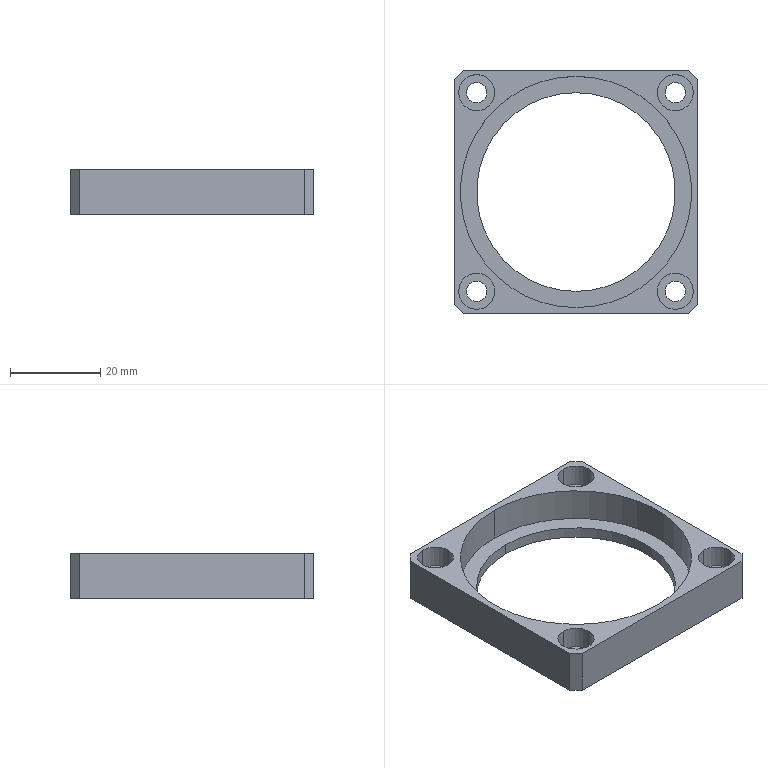NC program | NX | posted with a generic post | part box 54 x 54 x 10 mm
Whole program:
N10 G17 G21 G94 G90
(DRILLING , TOOL : D6A45)
N12 T07 M6
N14 G54
N16 G17 G0 G90 X22. Y-22. S5000 M3
N18 G43 Z30. H7
N20 G94 G81 G98 Z-1. F250. R3.
N22 Y22.
N24 X-22.
N26 X0. Y0.
N28 X-22. Y-22.
N30 G80
N32 G0 X-22. Y-22. Z30.
N34 M5
(DRILLING_COPY , TOOL : 4.5ZT)
N36 T14 M6
N38 G54
N40 G17 G0 G90 X22. Y-22. S2000 M3
N42 G43 Z30. H14
N44 G94 G83 G98 Z-12.852 F250. Q2. R3.
N46 Y22.
N48 X-22.
N50 X0. Y0.
N52 X-22. Y-22.
N54 G80
N56 G0 X-22. Y-22. Z30.
N58 M5
(HOLE_MILLING , TOOL : D6)
N60 T06 M6
N62 G54
N64 G17 G0 G90 X-22. Y22. S9500 M3
N66 G43 Z30. H6
N68 Z0.6
N70 G94 G3 X-21.5 Y21.5 R0.5 F1500.
N72 X-21. Y22. R0.5
N74 X-21. Y22. Z0.1 I-1. J0.
N76 X-21. Y22. Z-0.4 I-1. J0.
N78 X-21. Y22. Z-0.9 I-1. J0.
N80 X-21. Y22. Z-1.4 I-1. J0.
N82 X-21. Y22. Z-1.9 I-1. J0.
N84 X-21. Y22. Z-2.4 I-1. J0.
N86 X-21. Y22. Z-2.9 I-1. J0.
N88 X-21. Y22. Z-3.4 I-1. J0.
N90 X-21. Y22. Z-3.9 I-1. J0.
N92 X-21. Y22. Z-4.4 I-1. J0.
N94 X-21. Y22. Z-4.9 I-1. J0.
N96 X-21.691 Y22.951 Z-5. R1.
N98 X-22.951 Y22.309 R1.
N100 X-21.691 Y22.951 R-1.
N102 X-22.321 Y22.63 R0.5
N104 X-22. Y22. R0.5
N106 G0 Z30.
N108 X22.
N110 Z0.6
N112 G3 X22.5 Y21.5 R0.5
N114 X23. Y22. R0.5
N116 X23. Y22. Z0.1 I-1. J0.
N118 X23. Y22. Z-0.4 I-1. J0.
N120 X23. Y22. Z-0.9 I-1. J0.
N122 X23. Y22. Z-1.4 I-1. J0.
N124 X23. Y22. Z-1.9 I-1. J0.
N126 X23. Y22. Z-2.4 I-1. J0.
N128 X23. Y22. Z-2.9 I-1. J0.
N130 X23. Y22. Z-3.4 I-1. J0.
N132 X23. Y22. Z-3.9 I-1. J0.
N134 X23. Y22. Z-4.4 I-1. J0.
N136 X23. Y22. Z-4.9 I-1. J0.
N138 X22.309 Y22.951 Z-5. R1.
N140 X21.049 Y22.309 R1.
N142 X22.309 Y22.951 R-1.
N144 X21.679 Y22.63 R0.5
N146 X22. Y22. R0.5
N148 G0 Z30.
N150 Y-22.
N152 Z0.6
N154 G3 X22.5 Y-22.5 R0.5
N156 X23. Y-22. R0.5
N158 X23. Y-22. Z0.1 I-1. J0.
N160 X23. Y-22. Z-0.4 I-1. J0.
N162 X23. Y-22. Z-0.9 I-1. J0.
N164 X23. Y-22. Z-1.4 I-1. J0.
N166 X23. Y-22. Z-1.9 I-1. J0.
N168 X23. Y-22. Z-2.4 I-1. J0.
N170 X23. Y-22. Z-2.9 I-1. J0.
N172 X23. Y-22. Z-3.4 I-1. J0.
N174 X23. Y-22. Z-3.9 I-1. J0.
N176 X23. Y-22. Z-4.4 I-1. J0.
N178 X23. Y-22. Z-4.9 I-1. J0.
N180 X22.309 Y-21.049 Z-5. R1.
N182 X21.049 Y-21.691 R1.
N184 X22.309 Y-21.049 R-1.
N186 X21.679 Y-21.37 R0.5
N188 X22. Y-22. R0.5
N190 G0 Z30.
N192 X-22.
N194 Z0.6
N196 G3 X-21.5 Y-22.5 R0.5
N198 X-21. Y-22. R0.5
N200 X-21. Y-22. Z0.1 I-1. J0.
N202 X-21. Y-22. Z-0.4 I-1. J0.
N204 X-21. Y-22. Z-0.9 I-1. J0.
N206 X-21. Y-22. Z-1.4 I-1. J0.
N208 X-21. Y-22. Z-1.9 I-1. J0.
N210 X-21. Y-22. Z-2.4 I-1. J0.
N212 X-21. Y-22. Z-2.9 I-1. J0.
N214 X-21. Y-22. Z-3.4 I-1. J0.
N216 X-21. Y-22. Z-3.9 I-1. J0.
N218 X-21. Y-22. Z-4.4 I-1. J0.
N220 X-21. Y-22. Z-4.9 I-1. J0.
N222 X-21.691 Y-21.049 Z-5. R1.
N224 X-22.951 Y-21.691 R1.
N226 X-21.691 Y-21.049 R-1.
N228 X-22.321 Y-21.37 R0.5
N230 X-22. Y-22. R0.5
N232 G0 Z30.
N234 M5
(HOLE_MILLING_COPY , TOOL : D10)
N236 T10 M6
N238 G54
N240 G17 G0 G90 X0. Y0. S9500 M3
N242 G43 Z30. H10
N244 Z0.6
N246 G94 G3 X2.563 Y-2.563 R2.562 F2200.
N248 X5.125 Y0. R2.562
N250 X5.125 Y0. Z0.1 I-5.125 J0.
N252 X5.125 Y0. Z-0.4 I-5.125 J0.
N254 X5.125 Y0. Z-0.9 I-5.125 J0.
N256 X5.125 Y0. Z-1.4 I-5.125 J0.
N258 X5.125 Y0. Z-1.9 I-5.125 J0.
N260 X5.125 Y0. Z-2.4 I-5.125 J0.
N262 X5.125 Y0. Z-2.9 I-5.125 J0.
N264 X5.125 Y0. Z-3.4 I-5.125 J0.
N266 X5.125 Y0. Z-3.9 I-5.125 J0.
N268 X5.125 Y0. Z-4.4 I-5.125 J0.
N270 X5.125 Y0. Z-4.9 I-5.125 J0.
N272 X5.125 Y0. Z-5.4 I-5.125 J0.
N274 X5.125 Y0. Z-5.9 I-5.125 J0.
N276 X5.125 Y0. Z-6.4 I-5.125 J0.
N278 X5.125 Y0. Z-6.9 I-5.125 J0.
N280 X5.125 Y0. Z-7.4 I-5.125 J0.
N282 X1.584 Y4.874 Z-7.5 R5.125
N284 X-4.874 Y1.584 R5.125
N286 X1.584 Y4.874 R-5.125
N288 X-1.645 Y3.229 R2.563
N290 X0. Y0. R2.563
N292 G0 Z0.6
N294 G3 X5.125 Y-5.125 R5.125
N296 X10.25 Y0. R5.125
N298 X10.25 Y0. Z0.1 I-10.25 J0.
N300 X10.25 Y0. Z-0.4 I-10.25 J0.
N302 X10.25 Y0. Z-0.9 I-10.25 J0.
N304 X10.25 Y0. Z-1.4 I-10.25 J0.
N306 X10.25 Y0. Z-1.9 I-10.25 J0.
N308 X10.25 Y0. Z-2.4 I-10.25 J0.
N310 X10.25 Y0. Z-2.9 I-10.25 J0.
N312 X10.25 Y0. Z-3.4 I-10.25 J0.
N314 X10.25 Y0. Z-3.9 I-10.25 J0.
N316 X10.25 Y0. Z-4.4 I-10.25 J0.
N318 X10.25 Y0. Z-4.9 I-10.25 J0.
N320 X10.25 Y0. Z-5.4 I-10.25 J0.
N322 X10.25 Y0. Z-5.9 I-10.25 J0.
N324 X10.25 Y0. Z-6.4 I-10.25 J0.
N326 X10.25 Y0. Z-6.9 I-10.25 J0.
N328 X10.25 Y0. Z-7.4 I-10.25 J0.
N330 X3.167 Y9.748 Z-7.5 R10.25
N332 X-9.748 Y3.167 R10.25
N334 X3.167 Y9.748 R-10.25
N336 X-3.29 Y6.458 R5.125
N338 X0. Y0. R5.125
N340 G0 Z0.6
N342 G3 X7.688 Y-7.688 R7.688
N344 X15.375 Y0. R7.688
N346 X15.375 Y0. Z0.1 I-15.375 J0.
N348 X15.375 Y0. Z-0.4 I-15.375 J0.
N350 X15.375 Y0. Z-0.9 I-15.375 J0.
N352 X15.375 Y0. Z-1.4 I-15.375 J0.
N354 X15.375 Y0. Z-1.9 I-15.375 J0.
N356 X15.375 Y0. Z-2.4 I-15.375 J0.
N358 X15.375 Y0. Z-2.9 I-15.375 J0.
N360 X15.375 Y0. Z-3.4 I-15.375 J0.
N362 X15.375 Y0. Z-3.9 I-15.375 J0.
N364 X15.375 Y0. Z-4.4 I-15.375 J0.
N366 X15.375 Y0. Z-4.9 I-15.375 J0.
N368 X15.375 Y0. Z-5.4 I-15.375 J0.
N370 X15.375 Y0. Z-5.9 I-15.375 J0.
N372 X15.375 Y0. Z-6.4 I-15.375 J0.
N374 X15.375 Y0. Z-6.9 I-15.375 J0.
N376 X15.375 Y0. Z-7.4 I-15.375 J0.
N378 X4.751 Y14.622 Z-7.5 R15.375
N380 X-14.622 Y4.751 R15.375
N382 X4.751 Y14.622 R-15.375
N384 X-4.936 Y9.687 R7.688
N386 X0. Y0. R7.688
N388 G0 Z0.6
N390 G3 X10.25 Y-10.25 R10.25
N392 X20.5 Y0. R10.25
N394 X20.5 Y0. Z0.1 I-20.5 J0.
N396 X20.5 Y0. Z-0.4 I-20.5 J0.
N398 X20.5 Y0. Z-0.9 I-20.5 J0.
N400 X20.5 Y0. Z-1.4 I-20.5 J0.
N402 X20.5 Y0. Z-1.9 I-20.5 J0.
N404 X20.5 Y0. Z-2.4 I-20.5 J0.
N406 X20.5 Y0. Z-2.9 I-20.5 J0.
N408 X20.5 Y0. Z-3.4 I-20.5 J0.
N410 X20.5 Y0. Z-3.9 I-20.5 J0.
N412 X20.5 Y0. Z-4.4 I-20.5 J0.
N414 X20.5 Y0. Z-4.9 I-20.5 J0.
N416 X20.5 Y0. Z-5.4 I-20.5 J0.
N418 X20.5 Y0. Z-5.9 I-20.5 J0.
N420 X20.5 Y0. Z-6.4 I-20.5 J0.
N422 X20.5 Y0. Z-6.9 I-20.5 J0.
N424 X20.5 Y0. Z-7.4 I-20.5 J0.
N426 X6.335 Y19.497 Z-7.5 R20.5
N428 X-19.497 Y6.335 R20.5
N430 X6.335 Y19.497 R-20.5
N432 X-6.581 Y12.916 R10.25
N434 X0. Y0. R10.25
N436 G0 Z30.
(HOLE_MILLING_COPY_COPY , TOOL : D10)
N438 Z-6.9
N440 G3 X2.817 Y-2.817 R2.817
N442 X5.633 Y0. R2.817
N444 X5.633 Y0. Z-7.4 I-5.633 J0.
N446 X5.633 Y0. Z-7.9 I-5.633 J0.
N448 X5.633 Y0. Z-8.4 I-5.633 J0.
N450 X5.633 Y0. Z-8.9 I-5.633 J0.
N452 X5.633 Y0. Z-9.4 I-5.633 J0.
N454 X5.633 Y0. Z-9.9 I-5.633 J0.
N456 X1.741 Y5.358 Z-10. R5.633
N458 X-5.358 Y1.741 R5.633
N460 X1.741 Y5.358 R-5.633
N462 X-1.808 Y3.549 R2.817
N464 X0. Y0. R2.817
N466 G0 Z-6.9
N468 G3 X5.633 Y-5.633 R5.633
N470 X11.267 Y0. R5.633
N472 X11.267 Y0. Z-7.4 I-11.267 J0.
N474 X11.267 Y0. Z-7.9 I-11.267 J0.
N476 X11.267 Y0. Z-8.4 I-11.267 J0.
N478 X11.267 Y0. Z-8.9 I-11.267 J0.
N480 X11.267 Y0. Z-9.4 I-11.267 J0.
N482 X11.267 Y0. Z-9.9 I-11.267 J0.
N484 X3.482 Y10.715 Z-10. R11.267
N486 X-10.715 Y3.482 R11.267
N488 X3.482 Y10.715 R-11.267
N490 X-3.617 Y7.098 R5.633
N492 X0. Y0. R5.633
N494 G0 Z-6.9
N496 G3 X8.45 Y-8.45 R8.45
N498 X16.9 Y0. R8.45
N500 X16.9 Y0. Z-7.4 I-16.9 J0.
N502 X16.9 Y0. Z-7.9 I-16.9 J0.
N504 X16.9 Y0. Z-8.4 I-16.9 J0.
N506 X16.9 Y0. Z-8.9 I-16.9 J0.
N508 X16.9 Y0. Z-9.4 I-16.9 J0.
N510 X16.9 Y0. Z-9.9 I-16.9 J0.
N512 X5.222 Y16.073 Z-10. R16.9
N514 X-16.073 Y5.222 R16.9
N516 X5.222 Y16.073 R-16.9
N518 X-5.425 Y10.648 R8.45
N520 X0. Y0. R8.45
N522 G0 Z30.
(ZLEVEL_PROFILE , TOOL : D10)
N524 X2.109 Y-32.1
N526 Z1.5
N528 G1 X-25. Z0.079 F1000.
N530 X-25.554 Z0.05
N532 X-26.963 Y-31.74 Z-0.026
N534 X-28.215 Y-30.998 Z-0.102
N536 X-30.998 Y-28.215 Z-0.309
N538 X-31.74 Y-26.963 Z-0.385
N540 X-32.1 Y-25.554 Z-0.461
N542 Y-25. Z-0.49
N544 Y25. F2500.
N546 G2 X-30.606 Y28.606 R5.1
N548 G1 X-28.606 Y30.606
N550 G2 X-25. Y32.1 R5.1
N552 G1 X25.
N554 G2 X28.606 Y30.606 R5.1
N556 G1 X30.606 Y28.606
N558 G2 X32.1 Y25. R5.1
N560 G1 Y-25.
N562 G2 X30.606 Y-28.606 R5.1
N564 G1 X28.606 Y-30.606
N566 G2 X25. Y-32.1 R5.1
N568 G1 X-25.
N570 G2 X-28.606 Y-30.606 R5.1
N572 G1 X-30.606 Y-28.606
N574 G2 X-32.1 Y-25. R5.1
N576 G1 Y3.072 Z-0.98
N578 Y25.
N580 G2 X-30.606 Y28.606 R5.1
N582 G1 X-28.606 Y30.606
N584 G2 X-25. Y32.1 R5.1
N586 G1 X25.
N588 G2 X28.606 Y30.606 R5.1
N590 G1 X30.606 Y28.606
N592 G2 X32.1 Y25. R5.1
N594 G1 Y-25.
N596 G2 X30.606 Y-28.606 R5.1
N598 G1 X28.606 Y-30.606
N600 G2 X25. Y-32.1 R5.1
N602 G1 X-25.
N604 G2 X-28.606 Y-30.606 R5.1
N606 G1 X-30.606 Y-28.606
N608 G2 X-32.1 Y-25. R5.1
N610 G1 Y3.072 Z-1.47
N612 Y25.
N614 G2 X-30.606 Y28.606 R5.1
N616 G1 X-28.606 Y30.606
N618 G2 X-25. Y32.1 R5.1
N620 G1 X25.
N622 G2 X28.606 Y30.606 R5.1
N624 G1 X30.606 Y28.606
N626 G2 X32.1 Y25. R5.1
N628 G1 Y-25.
N630 G2 X30.606 Y-28.606 R5.1
N632 G1 X28.606 Y-30.606
N634 G2 X25. Y-32.1 R5.1
N636 G1 X-25.
N638 G2 X-28.606 Y-30.606 R5.1
N640 G1 X-30.606 Y-28.606
N642 G2 X-32.1 Y-25. R5.1
N644 G1 Y3.072 Z-1.96
N646 Y25.
N648 G2 X-30.606 Y28.606 R5.1
N650 G1 X-28.606 Y30.606
N652 G2 X-25. Y32.1 R5.1
N654 G1 X25.
N656 G2 X28.606 Y30.606 R5.1
N658 G1 X30.606 Y28.606
N660 G2 X32.1 Y25. R5.1
N662 G1 Y-25.
N664 G2 X30.606 Y-28.606 R5.1
N666 G1 X28.606 Y-30.606
N668 G2 X25. Y-32.1 R5.1
N670 G1 X-25.
N672 G2 X-28.606 Y-30.606 R5.1
N674 G1 X-30.606 Y-28.606
N676 G2 X-32.1 Y-25. R5.1
N678 G1 Y3.072 Z-2.45
N680 Y25.
N682 G2 X-30.606 Y28.606 R5.1
N684 G1 X-28.606 Y30.606
N686 G2 X-25. Y32.1 R5.1
N688 G1 X25.
N690 G2 X28.606 Y30.606 R5.1
N692 G1 X30.606 Y28.606
N694 G2 X32.1 Y25. R5.1
N696 G1 Y-25.
N698 G2 X30.606 Y-28.606 R5.1
N700 G1 X28.606 Y-30.606
N702 G2 X25. Y-32.1 R5.1
N704 G1 X-25.
N706 G2 X-28.606 Y-30.606 R5.1
N708 G1 X-30.606 Y-28.606
N710 G2 X-32.1 Y-25. R5.1
N712 G1 Y3.072 Z-2.94
N714 Y25.
N716 G2 X-30.606 Y28.606 R5.1
N718 G1 X-28.606 Y30.606
N720 G2 X-25. Y32.1 R5.1
N722 G1 X25.
N724 G2 X28.606 Y30.606 R5.1
N726 G1 X30.606 Y28.606
N728 G2 X32.1 Y25. R5.1
N730 G1 Y-25.
N732 G2 X30.606 Y-28.606 R5.1
N734 G1 X28.606 Y-30.606
N736 G2 X25. Y-32.1 R5.1
N738 G1 X-25.
N740 G2 X-28.606 Y-30.606 R5.1
N742 G1 X-30.606 Y-28.606
N744 G2 X-32.1 Y-25. R5.1
N746 G1 Y3.072 Z-3.43
N748 Y25.
N750 G2 X-30.606 Y28.606 R5.1
N752 G1 X-28.606 Y30.606
N754 G2 X-25. Y32.1 R5.1
N756 G1 X25.
N758 G2 X28.606 Y30.606 R5.1
N760 G1 X30.606 Y28.606
N762 G2 X32.1 Y25. R5.1
N764 G1 Y-25.
N766 G2 X30.606 Y-28.606 R5.1
N768 G1 X28.606 Y-30.606
N770 G2 X25. Y-32.1 R5.1
N772 G1 X-25.
N774 G2 X-28.606 Y-30.606 R5.1
N776 G1 X-30.606 Y-28.606
N778 G2 X-32.1 Y-25. R5.1
N780 G1 Y3.072 Z-3.92
N782 Y25.
N784 G2 X-30.606 Y28.606 R5.1
N786 G1 X-28.606 Y30.606
N788 G2 X-25. Y32.1 R5.1
N790 G1 X25.
N792 G2 X28.606 Y30.606 R5.1
N794 G1 X30.606 Y28.606
N796 G2 X32.1 Y25. R5.1
N798 G1 Y-25.
N800 G2 X30.606 Y-28.606 R5.1
N802 G1 X28.606 Y-30.606
N804 G2 X25. Y-32.1 R5.1
N806 G1 X-25.
N808 G2 X-28.606 Y-30.606 R5.1
N810 G1 X-30.606 Y-28.606
N812 G2 X-32.1 Y-25. R5.1
N814 G1 Y3.072 Z-4.41
N816 Y25.
N818 G2 X-30.606 Y28.606 R5.1
N820 G1 X-28.606 Y30.606
N822 G2 X-25. Y32.1 R5.1
N824 G1 X25.
N826 G2 X28.606 Y30.606 R5.1
N828 G1 X30.606 Y28.606
N830 G2 X32.1 Y25. R5.1
N832 G1 Y-25.
N834 G2 X30.606 Y-28.606 R5.1
N836 G1 X28.606 Y-30.606
N838 G2 X25. Y-32.1 R5.1
N840 G1 X-25.
N842 G2 X-28.606 Y-30.606 R5.1
N844 G1 X-30.606 Y-28.606
N846 G2 X-32.1 Y-25. R5.1
N848 G1 Y3.072 Z-4.9
N850 Y25.
N852 G2 X-30.606 Y28.606 R5.1
N854 G1 X-28.606 Y30.606
N856 G2 X-25. Y32.1 R5.1
N858 G1 X25.
N860 G2 X28.606 Y30.606 R5.1
N862 G1 X30.606 Y28.606
N864 G2 X32.1 Y25. R5.1
N866 G1 Y-25.
N868 G2 X30.606 Y-28.606 R5.1
N870 G1 X28.606 Y-30.606
N872 G2 X25. Y-32.1 R5.1
N874 G1 X-25.
N876 G2 X-28.606 Y-30.606 R5.1
N878 G1 X-30.606 Y-28.606
N880 G2 X-32.1 Y-25. R5.1
N882 G1 Y3.645 Z-5.4
N884 Y25.
N886 G2 X-30.606 Y28.606 R5.1
N888 G1 X-28.606 Y30.606
N890 G2 X-25. Y32.1 R5.1
N892 G1 X25.
N894 G2 X28.606 Y30.606 R5.1
N896 G1 X30.606 Y28.606
N898 G2 X32.1 Y25. R5.1
N900 G1 Y-25.
N902 G2 X30.606 Y-28.606 R5.1
N904 G1 X28.606 Y-30.606
N906 G2 X25. Y-32.1 R5.1
N908 G1 X-25.
N910 G2 X-28.606 Y-30.606 R5.1
N912 G1 X-30.606 Y-28.606
N914 G2 X-32.1 Y-25. R5.1
N916 G1 Y3.645 Z-5.9
N918 Y25.
N920 G2 X-30.606 Y28.606 R5.1
N922 G1 X-28.606 Y30.606
N924 G2 X-25. Y32.1 R5.1
N926 G1 X25.
N928 G2 X28.606 Y30.606 R5.1
N930 G1 X30.606 Y28.606
N932 G2 X32.1 Y25. R5.1
N934 G1 Y-25.
N936 G2 X30.606 Y-28.606 R5.1
N938 G1 X28.606 Y-30.606
N940 G2 X25. Y-32.1 R5.1
N942 G1 X-25.
N944 G2 X-28.606 Y-30.606 R5.1
N946 G1 X-30.606 Y-28.606
N948 G2 X-32.1 Y-25. R5.1
N950 G1 Y3.645 Z-6.4
N952 Y25.
N954 G2 X-30.606 Y28.606 R5.1
N956 G1 X-28.606 Y30.606
N958 G2 X-25. Y32.1 R5.1
N960 G1 X25.
N962 G2 X28.606 Y30.606 R5.1
N964 G1 X30.606 Y28.606
N966 G2 X32.1 Y25. R5.1
N968 G1 Y-25.
N970 G2 X30.606 Y-28.606 R5.1
N972 G1 X28.606 Y-30.606
N974 G2 X25. Y-32.1 R5.1
N976 G1 X-25.
N978 G2 X-28.606 Y-30.606 R5.1
N980 G1 X-30.606 Y-28.606
N982 G2 X-32.1 Y-25. R5.1
N984 G1 Y3.645 Z-6.9
N986 Y25.
N988 G2 X-30.606 Y28.606 R5.1
N990 G1 X-28.606 Y30.606
N992 G2 X-25. Y32.1 R5.1
N994 G1 X25.
N996 G2 X28.606 Y30.606 R5.1
N998 G1 X30.606 Y28.606
N1000 G2 X32.1 Y25. R5.1
N1002 G1 Y-25.
N1004 G2 X30.606 Y-28.606 R5.1
N1006 G1 X28.606 Y-30.606
N1008 G2 X25. Y-32.1 R5.1
N1010 G1 X-25.
N1012 G2 X-28.606 Y-30.606 R5.1
N1014 G1 X-30.606 Y-28.606
N1016 G2 X-32.1 Y-25. R5.1
N1018 G1 Y3.645 Z-7.4
N1020 Y25.
N1022 G2 X-30.606 Y28.606 R5.1
N1024 G1 X-28.606 Y30.606
N1026 G2 X-25. Y32.1 R5.1
N1028 G1 X25.
N1030 G2 X28.606 Y30.606 R5.1
N1032 G1 X30.606 Y28.606
N1034 G2 X32.1 Y25. R5.1
N1036 G1 Y-25.
N1038 G2 X30.606 Y-28.606 R5.1
N1040 G1 X28.606 Y-30.606
N1042 G2 X25. Y-32.1 R5.1
N1044 G1 X-25.
N1046 G2 X-28.606 Y-30.606 R5.1
N1048 G1 X-30.606 Y-28.606
N1050 G2 X-32.1 Y-25. R5.1
N1052 G1 Y3.072 Z-7.89
N1054 Y25.
N1056 G2 X-30.606 Y28.606 R5.1
N1058 G1 X-28.606 Y30.606
N1060 G2 X-25. Y32.1 R5.1
N1062 G1 X25.
N1064 G2 X28.606 Y30.606 R5.1
N1066 G1 X30.606 Y28.606
N1068 G2 X32.1 Y25. R5.1
N1070 G1 Y-25.
N1072 G2 X30.606 Y-28.606 R5.1
N1074 G1 X28.606 Y-30.606
N1076 G2 X25. Y-32.1 R5.1
N1078 G1 X-25.
N1080 G2 X-28.606 Y-30.606 R5.1
N1082 G1 X-30.606 Y-28.606
N1084 G2 X-32.1 Y-25. R5.1
N1086 G1 Y3.072 Z-8.38
N1088 Y25.
N1090 G2 X-30.606 Y28.606 R5.1
N1092 G1 X-28.606 Y30.606
N1094 G2 X-25. Y32.1 R5.1
N1096 G1 X25.
N1098 G2 X28.606 Y30.606 R5.1
N1100 G1 X30.606 Y28.606
N1102 G2 X32.1 Y25. R5.1
N1104 G1 Y-25.
N1106 G2 X30.606 Y-28.606 R5.1
N1108 G1 X28.606 Y-30.606
N1110 G2 X25. Y-32.1 R5.1
N1112 G1 X-25.
N1114 G2 X-28.606 Y-30.606 R5.1
N1116 G1 X-30.606 Y-28.606
N1118 G2 X-32.1 Y-25. R5.1
N1120 G1 Y3.072 Z-8.87
N1122 Y25.
N1124 G2 X-30.606 Y28.606 R5.1
N1126 G1 X-28.606 Y30.606
N1128 G2 X-25. Y32.1 R5.1
N1130 G1 X25.
N1132 G2 X28.606 Y30.606 R5.1
N1134 G1 X30.606 Y28.606
N1136 G2 X32.1 Y25. R5.1
N1138 G1 Y-25.
N1140 G2 X30.606 Y-28.606 R5.1
N1142 G1 X28.606 Y-30.606
N1144 G2 X25. Y-32.1 R5.1
N1146 G1 X-25.
N1148 G2 X-28.606 Y-30.606 R5.1
N1150 G1 X-30.606 Y-28.606
N1152 G2 X-32.1 Y-25. R5.1
N1154 G1 Y3.072 Z-9.36
N1156 Y25.
N1158 G2 X-30.606 Y28.606 R5.1
N1160 G1 X-28.606 Y30.606
N1162 G2 X-25. Y32.1 R5.1
N1164 G1 X25.
N1166 G2 X28.606 Y30.606 R5.1
N1168 G1 X30.606 Y28.606
N1170 G2 X32.1 Y25. R5.1
N1172 G1 Y-25.
N1174 G2 X30.606 Y-28.606 R5.1
N1176 G1 X28.606 Y-30.606
N1178 G2 X25. Y-32.1 R5.1
N1180 G1 X-25.
N1182 G2 X-28.606 Y-30.606 R5.1
N1184 G1 X-30.606 Y-28.606
N1186 G2 X-32.1 Y-25. R5.1
N1188 G1 Y3.072 Z-9.85
N1190 Y25.
N1192 G2 X-30.606 Y28.606 R5.1
N1194 G1 X-28.606 Y30.606
N1196 G2 X-25. Y32.1 R5.1
N1198 G1 X25.
N1200 G2 X28.606 Y30.606 R5.1
N1202 G1 X30.606 Y28.606
N1204 G2 X32.1 Y25. R5.1
N1206 G1 Y-25.
N1208 G2 X30.606 Y-28.606 R5.1
N1210 G1 X28.606 Y-30.606
N1212 G2 X25. Y-32.1 R5.1
N1214 G1 X-25.
N1216 G2 X-28.606 Y-30.606 R5.1
N1218 G1 X-30.606 Y-28.606
N1220 G2 X-32.1 Y-25. R5.1
N1222 G1 Y3.072
N1224 Z-8.35
N1226 G0 Z30.
N1228 M5
(ZLEVEL_PROFILE_COPY_COPY , TOOL : D10JING)
N1230 T11 M6
N1232 G54
N1234 G17 G0 G90 X-18.514 Y1.781 S9500 M3
N1236 G43 Z30. H11
N1238 Z-5.5
N1240 G94 G1 Z-7.5 F1000.
N1242 X-20.1 Y0.866
N1244 G3 X-20.6 Y0. R1.
N1246 X0. Y-20.6 R20.6 F1200.
N1248 X-20.6 Y0. R-20.6
N1250 X-20.1 Y-0.866 R1.
N1252 G1 X-18.514 Y-1.781
N1254 Z-5.5
N1256 G0 Z30.
(ZLEVEL_PROFILE_COPY_COPY_COPY , TOOL : D10JING)
N1258 X-14.892 Y1.794
N1260 Z-8.
N1262 G1 Z-10. F1000.
N1264 X-16.5 Y0.866
N1266 G3 X-17. Y0. R1.
N1268 X0. Y-17. R17. F1200.
N1270 X-17. Y0. R-17.
N1272 X-16.5 Y-0.866 R1.
N1274 G1 X-14.892 Y-1.794
N1276 Z-8.
N1278 G0 Z30.
N1280 M5
(PLANAR_MILL , TOOL : D6A45)
N1282 T07 M6
N1284 G54
N1286 G17 G0 G90 X21.134 Y19.4 S9500 M3
N1288 G43 Z30. H7
N1290 Z0.5
N1292 G94 G1 Z-1. F1250.
N1294 G3 X22. Y18.9 R1.
N1296 X25.1 Y22. R3.1
N1298 X22. Y18.9 R-3.1
N1300 X22.866 Y19.4 R1.
N1302 G1 Z0.5
N1304 G0 Z30.
N1306 X28.4 Y-24.134
N1308 Z0.5
N1310 G1 Z-1.
N1312 G3 X27.9 Y-25. R1.
N1314 G2 X27.636 Y-25.636 R0.9
N1316 G1 X25.636 Y-27.636
N1318 G2 X25. Y-27.9 R0.9
N1320 G1 X-25.
N1322 G2 X-25.636 Y-27.636 R0.9
N1324 G1 X-27.636 Y-25.636
N1326 G2 X-27.9 Y-25. R0.9
N1328 G1 Y25.
N1330 G2 X-27.636 Y25.636 R0.9
N1332 G1 X-25.636 Y27.636
N1334 G2 X-25. Y27.9 R0.9
N1336 G1 X25.
N1338 G2 X25.636 Y27.636 R0.9
N1340 G1 X27.636 Y25.636
N1342 G2 X27.9 Y25. R0.9
N1344 G1 Y-25.
N1346 G3 X28.4 Y-25.866 R1.
N1348 G1 Z0.5
N1350 G0 Z30.
N1352 X21.134 Y-24.6
N1354 Z0.5
N1356 G1 Z-1.
N1358 G3 X22. Y-25.1 R1.
N1360 X25.1 Y-22. R3.1
N1362 X22. Y-25.1 R-3.1
N1364 X22.866 Y-24.6 R1.
N1366 G1 Z0.5
N1368 G0 Z30.
N1370 X-22.866
N1372 Z0.5
N1374 G1 Z-1.
N1376 G3 X-22. Y-25.1 R1.
N1378 X-18.9 Y-22. R3.1
N1380 X-22. Y-25.1 R-3.1
N1382 X-21.134 Y-24.6 R1.
N1384 G1 Z0.5
N1386 G0 Z30.
N1388 X0.866 Y24.2
N1390 Z0.5
N1392 G1 Z-1.
N1394 G3 X0. Y24.7 R1.
N1396 X-24.7 Y0. R24.7
N1398 X0. Y24.7 R-24.7
N1400 X-0.866 Y24.2 R1.
N1402 G1 Z0.5
N1404 G0 Z30.
N1406 X-22.866 Y19.4
N1408 Z0.5
N1410 G1 Z-1.
N1412 G3 X-22. Y18.9 R1.
N1414 X-18.9 Y22. R3.1
N1416 X-22. Y18.9 R-3.1
N1418 X-21.134 Y19.4 R1.
N1420 G1 Z0.5
N1422 G0 Z30.
(PLANAR_MILL_COPY , TOOL : D6A45)
N1424 X0.866 Y20.6
N1426 Z-7.
N1428 G1 Z-8.5
N1430 G3 X0. Y21.1 R1.
N1432 X-21.1 Y0. R21.1
N1434 X0. Y21.1 R-21.1
N1436 X-0.866 Y20.6 R1.
N1438 G1 Z-7.
N1440 G0 Z30.
N1442 M5
(ZLEVEL_PROFILE_COPY , TOOL : D10JING)
N1444 T11 M6
N1446 G54
N1448 G17 G0 G90 X31.316 Y27.524 S9500 M3
N1450 G43 Z30. H11
N1452 Z1.5
N1454 G94 G1 X31.629 Y26.917 Z1.464 F1000.
N1456 X31.88 Y26.132 Z1.421
N1458 X32. Y25.316 Z1.378
N1460 Y-25. Z-1.259
N1462 Y-25.316 Z-1.276
N1464 X31.88 Y-26.132 Z-1.319
N1466 X31.629 Y-26.917 Z-1.362
N1468 X31.252 Y-27.65 Z-1.405
N1470 X30.759 Y-28.312 Z-1.449
N1472 X28.312 Y-30.759 Z-1.63
N1474 X27.65 Y-31.252 Z-1.673
N1476 X26.917 Y-31.629 Z-1.716
N1478 X26.132 Y-31.88 Z-1.76
N1480 X25.316 Y-32. Z-1.803
N1482 X-25. Z-4.44
N1484 X-25.316 Z-4.456
N1486 X-26.132 Y-31.88 Z-4.5
N1488 X-26.917 Y-31.629 Z-4.543
N1490 X-27.65 Y-31.252 Z-4.586
N1492 X-28.312 Y-30.759 Z-4.629
N1494 X-30.759 Y-28.312 Z-4.811
N1496 X-31.252 Y-27.65 Z-4.854
N1498 X-31.629 Y-26.917 Z-4.897
N1500 X-31.88 Y-26.132 Z-4.94
N1502 X-32. Y-25.316 Z-4.983
N1504 Y-25. Z-5.
N1506 Y25. F1200.
N1508 G2 X-30.536 Y28.536 R5.
N1510 G1 X-28.536 Y30.536
N1512 G2 X-25. Y32. R5.
N1514 G1 X25.
N1516 G2 X28.536 Y30.536 R5.
N1518 G1 X30.536 Y28.536
N1520 G2 X32. Y25. R5.
N1522 G1 Y-25.
N1524 G2 X30.536 Y-28.536 R5.
N1526 G1 X28.536 Y-30.536
N1528 G2 X25. Y-32. R5.
N1530 G1 X-25.
N1532 G2 X-28.536 Y-30.536 R5.
N1534 G1 X-30.536 Y-28.536
N1536 G2 X-32. Y-25. R5.
N1538 G1 Y24.973 Z-5.872
N1540 X-31.996 Y25.196 Z-5.876
N1542 X-31.982 Y25.418 Z-5.88
N1544 X-31.959 Y25.64 Z-5.884
N1546 X-31.925 Y25.861 Z-5.888
N1548 X-31.882 Y26.079 Z-5.892
N1550 X-31.829 Y26.296 Z-5.896
N1552 X-31.766 Y26.51 Z-5.9
N1554 X-31.694 Y26.721 Z-5.903
N1556 X-31.613 Y26.929 Z-5.907
N1558 X-31.522 Y27.133 Z-5.911
N1560 X-31.423 Y27.332 Z-5.915
N1562 X-31.314 Y27.527 Z-5.919
N1564 X-31.197 Y27.717 Z-5.923
N1566 X-31.072 Y27.902 Z-5.927
N1568 X-30.938 Y28.081 Z-5.931
N1570 X-30.797 Y28.253 Z-5.935
N1572 X-30.648 Y28.419 Z-5.938
N1574 X-30.492 Y28.579 Z-5.942
N1576 X-28.599 Y30.472 Z-5.989
N1578 X-28.44 Y30.628 Z-5.993
N1580 X-28.275 Y30.778 Z-5.997
N1582 X-28.103 Y30.92 Z-6.001
N1584 X-27.925 Y31.055 Z-6.005
N1586 X-27.741 Y31.181 Z-6.009
N1588 X-27.552 Y31.3 Z-6.012
N1590 X-27.358 Y31.409 Z-6.016
N1592 X-27.159 Y31.51 Z-6.02
N1594 X-26.956 Y31.602 Z-6.024
N1596 X-26.748 Y31.684 Z-6.028
N1598 X-26.538 Y31.758 Z-6.032
N1600 X-26.324 Y31.822 Z-6.036
N1602 X-26.108 Y31.876 Z-6.04
N1604 X-25.889 Y31.92 Z-6.044
N1606 X-25.669 Y31.955 Z-6.048
N1608 X-25.447 Y31.98 Z-6.051
N1610 X-25.224 Y31.995 Z-6.055
N1612 X-25.001 Y32. Z-6.059
N1614 X-24.778 Z-6.063
N1616 X24.971 Z-6.931
N1618 X25.194 Y31.996 Z-6.935
N1620 X25.417 Y31.983 Z-6.939
N1622 X25.639 Y31.959 Z-6.943
N1624 X25.859 Y31.926 Z-6.947
N1626 X26.078 Y31.882 Z-6.951
N1628 X26.295 Y31.829 Z-6.955
N1630 X26.509 Y31.767 Z-6.959
N1632 X26.72 Y31.695 Z-6.963
N1634 X26.928 Y31.613 Z-6.967
N1636 X27.132 Y31.523 Z-6.97
N1638 X27.331 Y31.423 Z-6.974
N1640 X27.526 Y31.315 Z-6.978
N1642 X27.716 Y31.198 Z-6.982
N1644 X27.901 Y31.073 Z-6.986
N1646 X28.079 Y30.939 Z-6.99
N1648 X28.252 Y30.798 Z-6.994
N1650 X28.418 Y30.649 Z-6.998
N1652 X28.578 Y30.493 Z-7.002
N1654 X30.471 Y28.6 Z-7.048
N1656 X30.627 Y28.441 Z-7.052
N1658 X30.777 Y28.276 Z-7.056
N1660 X30.92 Y28.104 Z-7.06
N1662 X31.054 Y27.926 Z-7.064
N1664 X31.181 Y27.743 Z-7.068
N1666 X31.299 Y27.554 Z-7.072
N1668 X31.408 Y27.359 Z-7.076
N1670 X31.509 Y27.16 Z-7.079
N1672 X31.601 Y26.957 Z-7.083
N1674 X31.684 Y26.75 Z-7.087
N1676 X31.757 Y26.539 Z-7.091
N1678 X31.821 Y26.325 Z-7.095
N1680 X31.875 Y26.109 Z-7.099
N1682 X31.92 Y25.89 Z-7.103
N1684 X31.955 Y25.67 Z-7.107
N1686 X31.98 Y25.448 Z-7.111
N1688 X31.995 Y25.226 Z-7.114
N1690 X32. Y25.003 Z-7.118
N1692 Y24.78 Z-7.122
N1694 Y3.14 Z-7.5
N1696 Y-25.
N1698 G2 X30.536 Y-28.536 R5.
N1700 G1 X28.536 Y-30.536
N1702 G2 X25. Y-32. R5.
N1704 G1 X-25.
N1706 G2 X-28.536 Y-30.536 R5.
N1708 G1 X-30.536 Y-28.536
N1710 G2 X-32. Y-25. R5.
N1712 G1 Y24.999 Z-8.373
N1714 X-31.995 Y25.222 Z-8.377
N1716 X-31.98 Y25.444 Z-8.381
N1718 X-31.955 Y25.666 Z-8.384
N1720 X-31.921 Y25.887 Z-8.388
N1722 X-31.876 Y26.105 Z-8.392
N1724 X-31.822 Y26.322 Z-8.396
N1726 X-31.758 Y26.536 Z-8.4
N1728 X-31.685 Y26.747 Z-8.404
N1730 X-31.602 Y26.954 Z-8.408
N1732 X-31.511 Y27.157 Z-8.412
N1734 X-31.41 Y27.356 Z-8.416
N1736 X-31.3 Y27.551 Z-8.419
N1738 X-31.182 Y27.74 Z-8.423
N1740 X-31.056 Y27.924 Z-8.427
N1742 X-30.921 Y28.102 Z-8.431
N1744 X-30.779 Y28.274 Z-8.435
N1746 X-30.629 Y28.44 Z-8.439
N1748 X-30.472 Y28.599 Z-8.443
N1750 X-28.578 Y30.493 Z-8.49
N1752 X-28.419 Y30.649 Z-8.494
N1754 X-28.253 Y30.798 Z-8.497
N1756 X-28.08 Y30.939 Z-8.501
N1758 X-27.901 Y31.072 Z-8.505
N1760 X-27.716 Y31.198 Z-8.509
N1762 X-27.526 Y31.315 Z-8.513
N1764 X-27.331 Y31.423 Z-8.517
N1766 X-27.132 Y31.523 Z-8.521
N1768 X-26.928 Y31.614 Z-8.525
N1770 X-26.72 Y31.695 Z-8.529
N1772 X-26.509 Y31.767 Z-8.532
N1774 X-26.294 Y31.83 Z-8.536
N1776 X-26.077 Y31.883 Z-8.54
N1778 X-25.858 Y31.926 Z-8.544
N1780 X-25.638 Y31.959 Z-8.548
N1782 X-25.416 Y31.983 Z-8.552
N1784 X-25.193 Y31.996 Z-8.556
N1786 X-24.97 Y32. Z-8.56
N1788 X24.805 Z-9.429
N1790 X25.029 Z-9.432
N1792 X25.252 Y31.994 Z-9.436
N1794 X25.474 Y31.977 Z-9.44
N1796 X25.696 Y31.951 Z-9.444
N1798 X25.916 Y31.915 Z-9.448
N1800 X26.135 Y31.87 Z-9.452
N1802 X26.351 Y31.814 Z-9.456
N1804 X26.564 Y31.749 Z-9.46
N1806 X26.775 Y31.674 Z-9.464
N1808 X26.982 Y31.591 Z-9.468
N1810 X27.184 Y31.498 Z-9.471
N1812 X27.383 Y31.396 Z-9.475
N1814 X27.577 Y31.285 Z-9.479
N1816 X27.765 Y31.166 Z-9.483
N1818 X27.949 Y31.038 Z-9.487
N1820 X28.126 Y30.902 Z-9.491
N1822 X28.297 Y30.759 Z-9.495
N1824 X28.461 Y30.608 Z-9.499
N1826 X28.62 Y30.451 Z-9.503
N1828 X30.514 Y28.557 Z-9.549
N1830 X30.669 Y28.397 Z-9.553
N1832 X30.817 Y28.23 Z-9.557
N1834 X30.957 Y28.056 Z-9.561
N1836 X31.09 Y27.876 Z-9.565
N1838 X31.214 Y27.691 Z-9.569
N1840 X31.33 Y27.5 Z-9.573
N1842 X31.437 Y27.305 Z-9.577
N1844 X31.536 Y27.104 Z-9.581
N1846 X31.625 Y26.9 Z-9.584
N1848 X31.705 Y26.691 Z-9.588
N1850 X31.776 Y26.48 Z-9.592
N1852 X31.837 Y26.265 Z-9.596
N1854 X31.889 Y26.048 Z-9.6
N1856 X31.931 Y25.829 Z-9.604
N1858 X31.963 Y25.608 Z-9.608
N1860 X31.985 Y25.386 Z-9.612
N1862 X31.997 Y25.163 Z-9.616
N1864 X32. Y24.94 Z-9.619
N1866 Y8.869 Z-9.9
N1868 Y-25.
N1870 G2 X30.536 Y-28.536 R5.
N1872 G1 X28.536 Y-30.536
N1874 G2 X25. Y-32. R5.
N1876 G1 X-25.
N1878 G2 X-28.536 Y-30.536 R5.
N1880 G1 X-30.536 Y-28.536
N1882 G2 X-32. Y-25. R5.
N1884 G1 Y25.
N1886 G2 X-30.536 Y28.536 R5.
N1888 G1 X-28.536 Y30.536
N1890 G2 X-25. Y32. R5.
N1892 G1 X25.
N1894 G2 X28.536 Y30.536 R5.
N1896 G1 X30.536 Y28.536
N1898 G2 X32. Y25. R5.
N1900 G1 Y8.869
N1902 Z-8.4
N1904 G0 Z30.
N1906 M5
N1908 M2